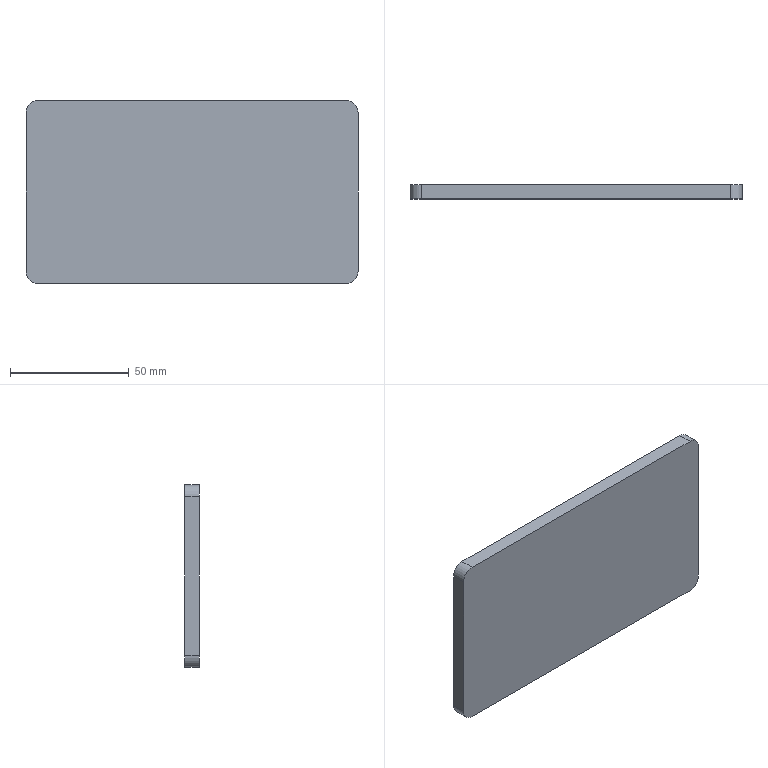Part | STEP file | WEAR-PLATE1_id182_x_t | 1 solid | 10 faces | box 140 x 6 x 77 mm | volume 64551 mm3 | plane 6 | cylinder 4 | commonest cylinder face diameters 10 x4
STEP:
#1=CARTESIAN_POINT('',(50.,-66.,160.));
#2=VERTEX_POINT('',#1);
#3=CARTESIAN_POINT('',(45.,-66.,155.));
#4=VERTEX_POINT('',#3);
#5=CARTESIAN_POINT('',(45.,-66.,160.));
#6=DIRECTION('',(0.,1.,0.));
#7=DIRECTION('',(0.,0.,1.));
#8=AXIS2_PLACEMENT_3D('',#5,#6,#7);
#9=CIRCLE('',#8,5.);
#10=EDGE_CURVE('',#2,#4,#9,.T.);
#11=ORIENTED_EDGE('',*,*,#10,.F.);
#12=CARTESIAN_POINT('',(50.,-66.,227.));
#13=VERTEX_POINT('',#12);
#14=CARTESIAN_POINT('',(50.,-66.,227.));
#15=DIRECTION('',(0.,0.,-1.));
#16=VECTOR('',#15,1.);
#17=LINE('',#14,#16);
#18=EDGE_CURVE('',#13,#2,#17,.T.);
#19=ORIENTED_EDGE('',*,*,#18,.F.);
#20=CARTESIAN_POINT('',(45.,-66.,232.));
#21=VERTEX_POINT('',#20);
#22=CARTESIAN_POINT('',(45.,-66.,227.));
#23=DIRECTION('',(0.,1.,0.));
#24=DIRECTION('',(0.,0.,1.));
#25=AXIS2_PLACEMENT_3D('',#22,#23,#24);
#26=CIRCLE('',#25,5.);
#27=EDGE_CURVE('',#21,#13,#26,.T.);
#28=ORIENTED_EDGE('',*,*,#27,.F.);
#29=CARTESIAN_POINT('',(-85.,-66.,232.));
#30=VERTEX_POINT('',#29);
#31=CARTESIAN_POINT('',(-85.,-66.,232.));
#32=DIRECTION('',(1.,0.,0.));
#33=VECTOR('',#32,1.);
#34=LINE('',#31,#33);
#35=EDGE_CURVE('',#30,#21,#34,.T.);
#36=ORIENTED_EDGE('',*,*,#35,.F.);
#37=CARTESIAN_POINT('',(-90.,-66.,227.));
#38=VERTEX_POINT('',#37);
#39=CARTESIAN_POINT('',(-85.,-66.,227.));
#40=DIRECTION('',(0.,1.,0.));
#41=DIRECTION('',(0.,0.,1.));
#42=AXIS2_PLACEMENT_3D('',#39,#40,#41);
#43=CIRCLE('',#42,5.);
#44=EDGE_CURVE('',#38,#30,#43,.T.);
#45=ORIENTED_EDGE('',*,*,#44,.F.);
#46=CARTESIAN_POINT('',(-90.,-66.,160.));
#47=VERTEX_POINT('',#46);
#48=CARTESIAN_POINT('',(-90.,-66.,160.));
#49=DIRECTION('',(0.,0.,1.));
#50=VECTOR('',#49,1.);
#51=LINE('',#48,#50);
#52=EDGE_CURVE('',#47,#38,#51,.T.);
#53=ORIENTED_EDGE('',*,*,#52,.F.);
#54=CARTESIAN_POINT('',(-85.,-66.,155.));
#55=VERTEX_POINT('',#54);
#56=CARTESIAN_POINT('',(-85.,-66.,160.));
#57=DIRECTION('',(0.,1.,0.));
#58=DIRECTION('',(0.,0.,1.));
#59=AXIS2_PLACEMENT_3D('',#56,#57,#58);
#60=CIRCLE('',#59,5.);
#61=EDGE_CURVE('',#55,#47,#60,.T.);
#62=ORIENTED_EDGE('',*,*,#61,.F.);
#63=CARTESIAN_POINT('',(45.,-66.,155.));
#64=DIRECTION('',(-1.,0.,0.));
#65=VECTOR('',#64,1.);
#66=LINE('',#63,#65);
#67=EDGE_CURVE('',#4,#55,#66,.T.);
#68=ORIENTED_EDGE('',*,*,#67,.F.);
#69=EDGE_LOOP('',(#11,#19,#28,#36,#45,#53,#62,#68));
#70=FACE_OUTER_BOUND('',#69,.T.);
#71=CARTESIAN_POINT('',(-200.,-66.,-275.));
#72=DIRECTION('',(0.,1.,0.));
#73=DIRECTION('',(0.,0.,1.));
#74=AXIS2_PLACEMENT_3D('',#71,#72,#73);
#75=PLANE('',#74);
#76=ADVANCED_FACE('',(#70),#75,.F.);
#77=CARTESIAN_POINT('',(-85.,-60.,155.));
#78=VERTEX_POINT('',#77);
#79=CARTESIAN_POINT('',(-85.,-66.,155.));
#80=DIRECTION('',(0.,1.,0.));
#81=VECTOR('',#80,1.);
#82=LINE('',#79,#81);
#83=EDGE_CURVE('',#55,#78,#82,.T.);
#84=ORIENTED_EDGE('',*,*,#83,.F.);
#85=ORIENTED_EDGE('',*,*,#61,.T.);
#86=CARTESIAN_POINT('',(-90.,-60.,160.));
#87=VERTEX_POINT('',#86);
#88=CARTESIAN_POINT('',(-90.,-66.,160.));
#89=DIRECTION('',(0.,-1.,0.));
#90=VECTOR('',#89,1.);
#91=LINE('',#88,#90);
#92=EDGE_CURVE('',#87,#47,#91,.T.);
#93=ORIENTED_EDGE('',*,*,#92,.F.);
#94=CARTESIAN_POINT('',(-85.,-60.,160.));
#95=DIRECTION('',(0.,-1.,0.));
#96=DIRECTION('',(0.,0.,1.));
#97=AXIS2_PLACEMENT_3D('',#94,#95,#96);
#98=CIRCLE('',#97,5.);
#99=EDGE_CURVE('',#87,#78,#98,.T.);
#100=ORIENTED_EDGE('',*,*,#99,.T.);
#101=EDGE_LOOP('',(#84,#85,#93,#100));
#102=FACE_OUTER_BOUND('',#101,.T.);
#103=CARTESIAN_POINT('',(-85.,-66.,160.));
#104=DIRECTION('',(0.,1.,0.));
#105=DIRECTION('',(0.,0.,1.));
#106=AXIS2_PLACEMENT_3D('',#103,#104,#105);
#107=CYLINDRICAL_SURFACE('',#106,5.);
#108=ADVANCED_FACE('',(#102),#107,.T.);
#109=CARTESIAN_POINT('',(45.,-60.,155.));
#110=VERTEX_POINT('',#109);
#111=CARTESIAN_POINT('',(45.,-66.,155.));
#112=DIRECTION('',(0.,1.,0.));
#113=VECTOR('',#112,1.);
#114=LINE('',#111,#113);
#115=EDGE_CURVE('',#4,#110,#114,.T.);
#116=ORIENTED_EDGE('',*,*,#115,.F.);
#117=ORIENTED_EDGE('',*,*,#67,.T.);
#118=ORIENTED_EDGE('',*,*,#83,.T.);
#119=CARTESIAN_POINT('',(-80.,-60.,155.));
#120=DIRECTION('',(1.,0.,0.));
#121=VECTOR('',#120,1.);
#122=LINE('',#119,#121);
#123=EDGE_CURVE('',#78,#110,#122,.T.);
#124=ORIENTED_EDGE('',*,*,#123,.T.);
#125=EDGE_LOOP('',(#116,#117,#118,#124));
#126=FACE_OUTER_BOUND('',#125,.T.);
#127=CARTESIAN_POINT('',(45.,-66.,155.));
#128=DIRECTION('',(0.,0.,-1.));
#129=DIRECTION('',(-1.,0.,0.));
#130=AXIS2_PLACEMENT_3D('',#127,#128,#129);
#131=PLANE('',#130);
#132=ADVANCED_FACE('',(#126),#131,.T.);
#133=CARTESIAN_POINT('',(50.,-60.,160.));
#134=VERTEX_POINT('',#133);
#135=CARTESIAN_POINT('',(50.,-66.,160.));
#136=DIRECTION('',(0.,1.,0.));
#137=VECTOR('',#136,1.);
#138=LINE('',#135,#137);
#139=EDGE_CURVE('',#2,#134,#138,.T.);
#140=ORIENTED_EDGE('',*,*,#139,.F.);
#141=ORIENTED_EDGE('',*,*,#10,.T.);
#142=ORIENTED_EDGE('',*,*,#115,.T.);
#143=CARTESIAN_POINT('',(45.,-60.,160.));
#144=DIRECTION('',(0.,-1.,0.));
#145=DIRECTION('',(0.,0.,1.));
#146=AXIS2_PLACEMENT_3D('',#143,#144,#145);
#147=CIRCLE('',#146,5.);
#148=EDGE_CURVE('',#110,#134,#147,.T.);
#149=ORIENTED_EDGE('',*,*,#148,.T.);
#150=EDGE_LOOP('',(#140,#141,#142,#149));
#151=FACE_OUTER_BOUND('',#150,.T.);
#152=CARTESIAN_POINT('',(45.,-66.,160.));
#153=DIRECTION('',(0.,1.,0.));
#154=DIRECTION('',(0.,0.,1.));
#155=AXIS2_PLACEMENT_3D('',#152,#153,#154);
#156=CYLINDRICAL_SURFACE('',#155,5.);
#157=ADVANCED_FACE('',(#151),#156,.T.);
#158=CARTESIAN_POINT('',(50.,-60.,227.));
#159=VERTEX_POINT('',#158);
#160=CARTESIAN_POINT('',(50.,-66.,227.));
#161=DIRECTION('',(0.,1.,0.));
#162=VECTOR('',#161,1.);
#163=LINE('',#160,#162);
#164=EDGE_CURVE('',#13,#159,#163,.T.);
#165=ORIENTED_EDGE('',*,*,#164,.F.);
#166=ORIENTED_EDGE('',*,*,#18,.T.);
#167=ORIENTED_EDGE('',*,*,#139,.T.);
#168=CARTESIAN_POINT('',(50.,-60.,-43.));
#169=DIRECTION('',(0.,0.,1.));
#170=VECTOR('',#169,1.);
#171=LINE('',#168,#170);
#172=EDGE_CURVE('',#134,#159,#171,.T.);
#173=ORIENTED_EDGE('',*,*,#172,.T.);
#174=EDGE_LOOP('',(#165,#166,#167,#173));
#175=FACE_OUTER_BOUND('',#174,.T.);
#176=CARTESIAN_POINT('',(50.,-66.,227.));
#177=DIRECTION('',(1.,0.,0.));
#178=DIRECTION('',(0.,0.,-1.));
#179=AXIS2_PLACEMENT_3D('',#176,#177,#178);
#180=PLANE('',#179);
#181=ADVANCED_FACE('',(#175),#180,.T.);
#182=CARTESIAN_POINT('',(45.,-60.,232.));
#183=VERTEX_POINT('',#182);
#184=CARTESIAN_POINT('',(45.,-66.,232.));
#185=DIRECTION('',(0.,1.,0.));
#186=VECTOR('',#185,1.);
#187=LINE('',#184,#186);
#188=EDGE_CURVE('',#21,#183,#187,.T.);
#189=ORIENTED_EDGE('',*,*,#188,.F.);
#190=ORIENTED_EDGE('',*,*,#27,.T.);
#191=ORIENTED_EDGE('',*,*,#164,.T.);
#192=CARTESIAN_POINT('',(45.,-60.,227.));
#193=DIRECTION('',(0.,-1.,0.));
#194=DIRECTION('',(0.,0.,1.));
#195=AXIS2_PLACEMENT_3D('',#192,#193,#194);
#196=CIRCLE('',#195,5.);
#197=EDGE_CURVE('',#159,#183,#196,.T.);
#198=ORIENTED_EDGE('',*,*,#197,.T.);
#199=EDGE_LOOP('',(#189,#190,#191,#198));
#200=FACE_OUTER_BOUND('',#199,.T.);
#201=CARTESIAN_POINT('',(45.,-66.,227.));
#202=DIRECTION('',(0.,1.,0.));
#203=DIRECTION('',(0.,0.,1.));
#204=AXIS2_PLACEMENT_3D('',#201,#202,#203);
#205=CYLINDRICAL_SURFACE('',#204,5.);
#206=ADVANCED_FACE('',(#200),#205,.T.);
#207=CARTESIAN_POINT('',(-85.,-60.,232.));
#208=VERTEX_POINT('',#207);
#209=CARTESIAN_POINT('',(-85.,-66.,232.));
#210=DIRECTION('',(0.,1.,0.));
#211=VECTOR('',#210,1.);
#212=LINE('',#209,#211);
#213=EDGE_CURVE('',#30,#208,#212,.T.);
#214=ORIENTED_EDGE('',*,*,#213,.F.);
#215=ORIENTED_EDGE('',*,*,#35,.T.);
#216=ORIENTED_EDGE('',*,*,#188,.T.);
#217=CARTESIAN_POINT('',(-80.,-60.,232.));
#218=DIRECTION('',(-1.,0.,0.));
#219=VECTOR('',#218,1.);
#220=LINE('',#217,#219);
#221=EDGE_CURVE('',#183,#208,#220,.T.);
#222=ORIENTED_EDGE('',*,*,#221,.T.);
#223=EDGE_LOOP('',(#214,#215,#216,#222));
#224=FACE_OUTER_BOUND('',#223,.T.);
#225=CARTESIAN_POINT('',(-85.,-66.,232.));
#226=DIRECTION('',(0.,0.,1.));
#227=DIRECTION('',(1.,0.,0.));
#228=AXIS2_PLACEMENT_3D('',#225,#226,#227);
#229=PLANE('',#228);
#230=ADVANCED_FACE('',(#224),#229,.T.);
#231=CARTESIAN_POINT('',(-90.,-60.,227.));
#232=VERTEX_POINT('',#231);
#233=CARTESIAN_POINT('',(-90.,-66.,227.));
#234=DIRECTION('',(0.,1.,0.));
#235=VECTOR('',#234,1.);
#236=LINE('',#233,#235);
#237=EDGE_CURVE('',#38,#232,#236,.T.);
#238=ORIENTED_EDGE('',*,*,#237,.F.);
#239=ORIENTED_EDGE('',*,*,#44,.T.);
#240=ORIENTED_EDGE('',*,*,#213,.T.);
#241=CARTESIAN_POINT('',(-85.,-60.,227.));
#242=DIRECTION('',(0.,-1.,0.));
#243=DIRECTION('',(0.,0.,1.));
#244=AXIS2_PLACEMENT_3D('',#241,#242,#243);
#245=CIRCLE('',#244,5.);
#246=EDGE_CURVE('',#208,#232,#245,.T.);
#247=ORIENTED_EDGE('',*,*,#246,.T.);
#248=EDGE_LOOP('',(#238,#239,#240,#247));
#249=FACE_OUTER_BOUND('',#248,.T.);
#250=CARTESIAN_POINT('',(-85.,-66.,227.));
#251=DIRECTION('',(0.,1.,0.));
#252=DIRECTION('',(0.,0.,1.));
#253=AXIS2_PLACEMENT_3D('',#250,#251,#252);
#254=CYLINDRICAL_SURFACE('',#253,5.);
#255=ADVANCED_FACE('',(#249),#254,.T.);
#256=ORIENTED_EDGE('',*,*,#92,.T.);
#257=ORIENTED_EDGE('',*,*,#52,.T.);
#258=ORIENTED_EDGE('',*,*,#237,.T.);
#259=CARTESIAN_POINT('',(-90.,-60.,-43.));
#260=DIRECTION('',(0.,0.,-1.));
#261=VECTOR('',#260,1.);
#262=LINE('',#259,#261);
#263=EDGE_CURVE('',#232,#87,#262,.T.);
#264=ORIENTED_EDGE('',*,*,#263,.T.);
#265=EDGE_LOOP('',(#256,#257,#258,#264));
#266=FACE_OUTER_BOUND('',#265,.T.);
#267=CARTESIAN_POINT('',(-90.,-66.,160.));
#268=DIRECTION('',(-1.,0.,0.));
#269=DIRECTION('',(0.,0.,1.));
#270=AXIS2_PLACEMENT_3D('',#267,#268,#269);
#271=PLANE('',#270);
#272=ADVANCED_FACE('',(#266),#271,.T.);
#273=ORIENTED_EDGE('',*,*,#246,.F.);
#274=ORIENTED_EDGE('',*,*,#221,.F.);
#275=ORIENTED_EDGE('',*,*,#197,.F.);
#276=ORIENTED_EDGE('',*,*,#172,.F.);
#277=ORIENTED_EDGE('',*,*,#148,.F.);
#278=ORIENTED_EDGE('',*,*,#123,.F.);
#279=ORIENTED_EDGE('',*,*,#99,.F.);
#280=ORIENTED_EDGE('',*,*,#263,.F.);
#281=EDGE_LOOP('',(#273,#274,#275,#276,#277,#278,#279,#280));
#282=FACE_OUTER_BOUND('',#281,.T.);
#283=CARTESIAN_POINT('',(-80.,-60.,-43.));
#284=DIRECTION('',(0.,-1.,0.));
#285=DIRECTION('',(0.,0.,-1.));
#286=AXIS2_PLACEMENT_3D('',#283,#284,#285);
#287=PLANE('',#286);
#288=ADVANCED_FACE('',(#282),#287,.F.);
#289=CLOSED_SHELL('',(#76,#108,#132,#157,#181,#206,#230,#255,#272,#288));
#290=MANIFOLD_SOLID_BREP('',#289);
#291=(LENGTH_UNIT()NAMED_UNIT(*)SI_UNIT(.MILLI.,.METRE.));
#292=UNCERTAINTY_MEASURE_WITH_UNIT(LENGTH_MEASURE(0.00002),#291,'','');
#293=(NAMED_UNIT(*)PLANE_ANGLE_UNIT()SI_UNIT($,.RADIAN.));
#294=PLANE_ANGLE_MEASURE_WITH_UNIT(PLANE_ANGLE_MEASURE(0.01745),#293);
#295=DIMENSIONAL_EXPONENTS(0.,0.,0.,0.,0.,0.,0.);
#296=(CONVERSION_BASED_UNIT('DEGREE',#294)NAMED_UNIT(#295)PLANE_ANGLE_UNIT());
#297=(NAMED_UNIT(*)SI_UNIT($,.STERADIAN.)SOLID_ANGLE_UNIT());
#298=(GEOMETRIC_REPRESENTATION_CONTEXT(3)GLOBAL_UNCERTAINTY_ASSIGNED_CONTEXT((#292))GLOBAL_UNIT_ASSIGNED_CONTEXT((#291,#296,#297))REPRESENTATION_CONTEXT('',''));
#299=ADVANCED_BREP_SHAPE_REPRESENTATION('',(#290),#298);